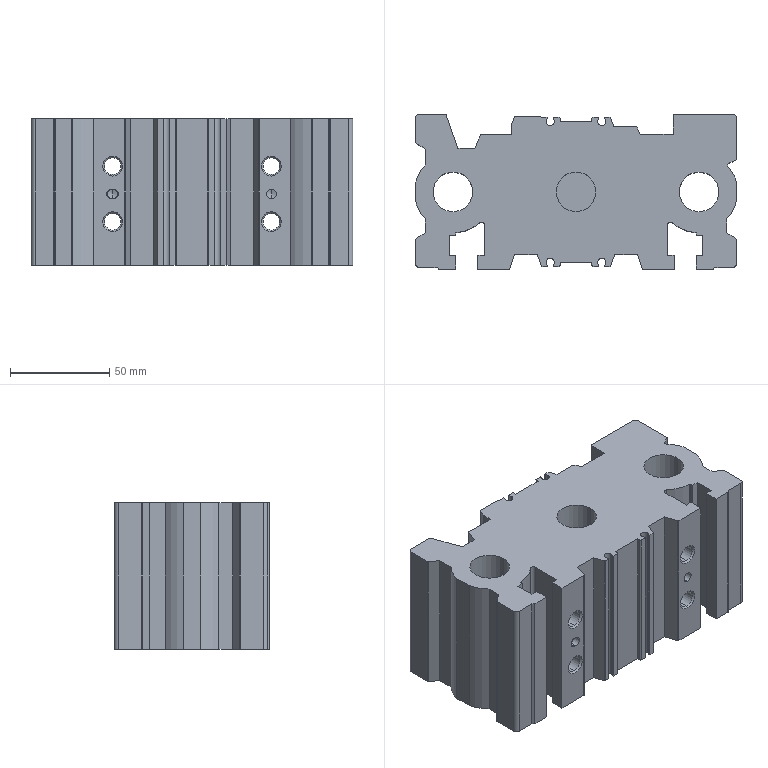Part | 1 solid | 236 faces | box 162 x 78 x 74 mm | volume 575326 mm3 | plane 109 | cylinder 99 | cone 28 | commonest cylinder face diameters 1 x22 8.376 x16 5 x13 4.2 x12 8.6 x8 11.445 x8